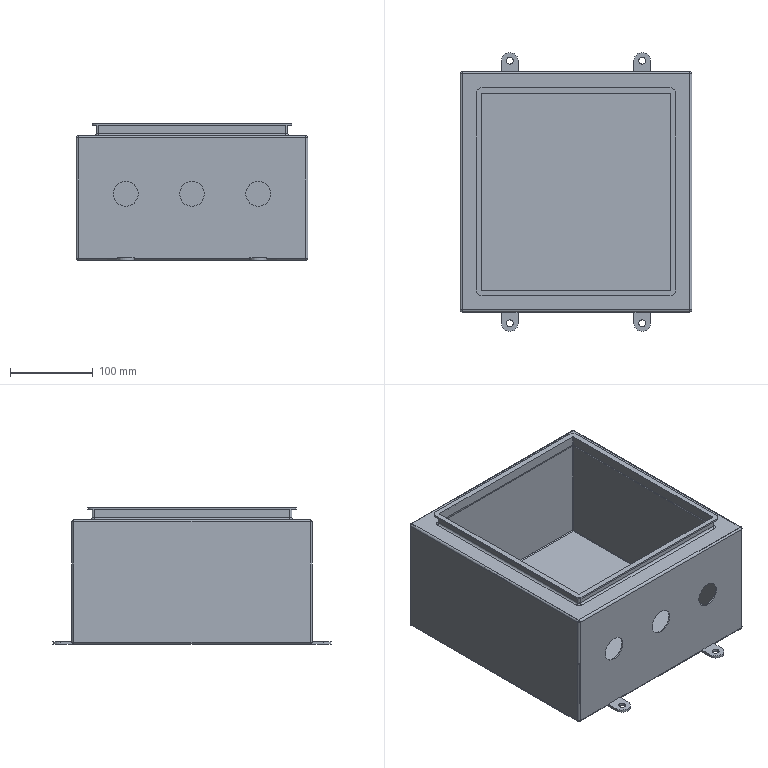Part | SolidWorks | features ICE 4, Fillet 2, Extrusion 1, Shell 1 | 1 solid | 132 faces | box 280 x 337 x 164.57 mm | volume 438435 mm3 | cylinder 62 | plane 46 | sphere 16 | torus 8 | commonest cylinder face diameters 4.8 x20 1.8 x16 8.2 x8 30 x6 7.8 x4 14.8 x4